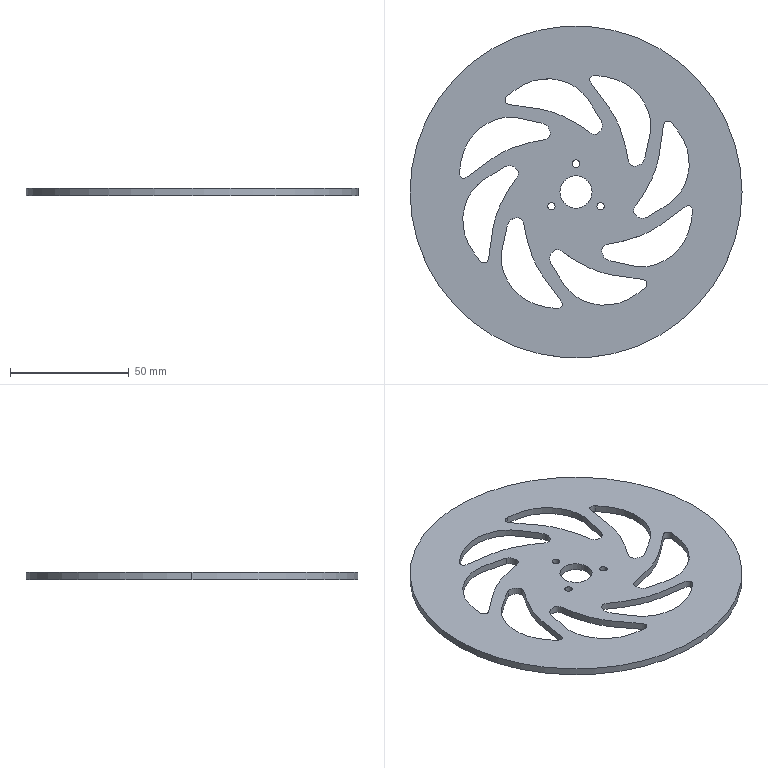Part | SolidWorks | features Extrusion 1, ICE 1 | 1 solid | 28 faces | box 140 x 140 x 3 mm | volume 34568 mm3 | spline 16 | cylinder 10 | plane 2 | commonest cylinder face diameters 3.141 x6 13.612 x2 140 x2